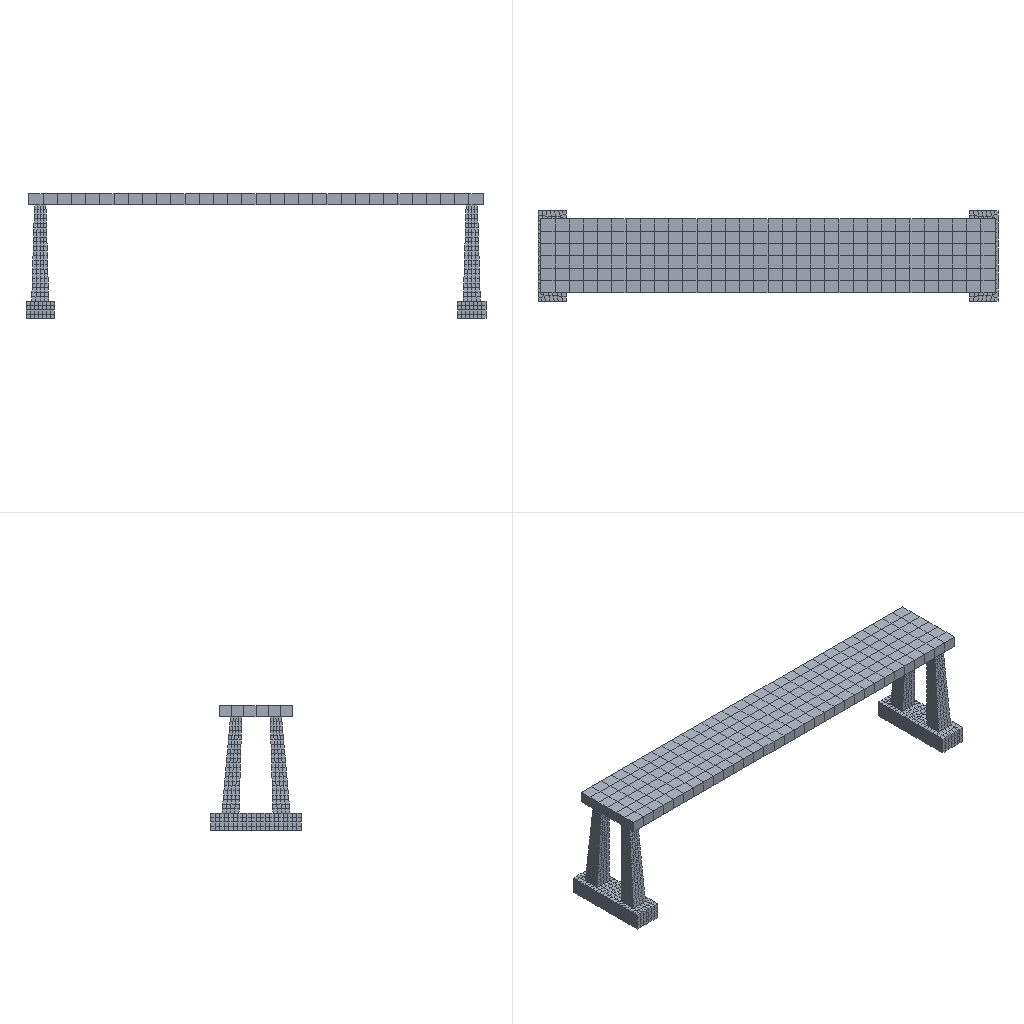Simulation study | ansys workbench
Set-up summary:
category,name,step,type,value,unit,region
solver,ansys_workbench
units,mm-N-s-tonne (MPa),,stated,"/units,MPA"
analysis,LS1,,static
load_step,LS1,LS1,static,nsubst=1; time=1
mesh,nodes,,,14374
mesh,elements,,,2852
element_type,SOLID186,,,2484
element_type,SURF154,,,192
element_type,TARGE170,,,88
element_type,CONTA174,,,88
material,steel,,E,210000,tonne s^-2 mm^-1
material,steel,,nu,0.3
material,steel,,density,7.85e-09,tonne mm^-3
load,Define Force Using Surface Effect Elements,LS1,surface-effect pres face 3,-0.09615,,SURF154 #8
bc,Fixed Supports,model,fixed,[dofs=ALL],,_FIXEDSU
contact,Contact Region,,bonded (always),element=CONTA174
contact,Contact Region 2,,bonded (always),element=CONTA174
named_set,_FIXEDSU,,node,821
Ansys APDL input file, long lists of numbers shortened:
/batch
/config,noeldb,1     ! force off writing results to database
*get,_wallstrt,active,,time,wall
! ANSYS input file written by Workbench version 2023 R1
! File used for geometry attach:
/title,wbnew--Static Structural (A5)
! ****** Begin Custom Load Command Snippet ******
/COM, ACT Extensions:
/COM,     LSDYNA, 2023.1
/COM,/COM,     ANSYSMotion, 2023.1
/COM,
! ****** End   Custom Load Command Snippet ******
*DIM,_wb_ProjectScratch_dir,string,248
_wb_ProjectScratch_dir(1) = ''
*DIM,_wb_SolverFiles_dir,string,248
_wb_SolverFiles_dir(1) = ''
*DIM,_wb_userfiles_dir,string,248
_wb_userfiles_dir(1) = ''
/com,--- Data in consistent NMM units. See Solving Units in the help system for more information.
/units,MPA
/nopr
/wb,file,start              !  signify a WB generated input file
/prep7
! Turn off shape checking because checks already performed inside WB mesher.
! See help system for more information.
SHPP,OFF,,NOWARN
/nolist
etcon,set             ! allow ANSYS to choose best KEYOP's for 180x elements, resets any applicable keyopt to MAPDL defaults
/com,*********** Nodes for the whole assembly ***********
nblock,3,,15811
(1i9,3e20.9e3)
        1     5.000000000E+02     1.450000000E+04     2.000000000E+04
! (14373 more lines like these left out)
-1
/wb,elem,start            !  set before creation of elements
/com,*********** Elements for Body 1 "longmendiao" ***********
et,1,186
keyo,1,2,1          ! set full integration on SOLID186
eblock,19,solid,,1148
(19i9)
        1        1        1        1        0        0        0        0       20        0      193     3225     3224     3193     3194     3322     3321     3290     3291
! (2295 more lines like these left out)
-1
/com,*********** Elements for Body 2 "longmendiao" ***********
et,2,186
keyo,2,2,1          ! set full integration on SOLID186
eblock,19,solid,,192
(19i9)
        2        2        2        2        0        0        0        0       20        0        1      393      459      461      395      394      460      462      396
! (383 more lines like these left out)
-1
/com,*********** Elements for Body 3 "longmendiao" ***********
et,3,186
keyo,3,2,1          ! set full integration on SOLID186
eblock,19,solid,,1144
(19i9)
        3        3        3        3        0        0        0        0       20        0     1341     9649     9648     9611     9610     9745     9744     9707     9706
! (2287 more lines like these left out)
-1
/wb,elem,end               !  done creating elements
/com,*********** Send User Defined Coordinate System(s) ***********
csys,0
toffst,273.15,  ! Temperature offset from absolute zero
/com,*********** Set Reference Temperature ***********
tref,22.
/wb,mat,start              !  starting to send materials
/com,*********** Send Materials ***********
MP,DENS,1,7.85e-09,	! tonne mm^-3
MP,EX,1,210000,	! tonne s^-2 mm^-1
MP,NUXY,1,0.3,
MP,DENS,2,7.85e-09,	! tonne mm^-3
MP,EX,2,210000,	! tonne s^-2 mm^-1
MP,NUXY,2,0.3,
MP,DENS,3,7.85e-09,	! tonne mm^-3
MP,EX,3,210000,	! tonne s^-2 mm^-1
MP,NUXY,3,0.3,
/wb,mat,end                !  done sending materials
!************************* Model Summary ********************
!longmendiao,	steel,	matid,	1
!longmendiao,	steel,	matid,	2
!longmendiao,	steel,	matid,	3
!************************* End Model Summary ********************
! get the diagonal of the bounding box. Needed later for other things
*get,_xmin,node,,mnloc,x
*get,_ymin,node,,mnloc,y
*get,_zmin,node,,mnloc,z
*get,_xmax,node,,mxloc,x
*get,_ymax,node,,mxloc,y
*get,_zmax,node,,mxloc,z
_ASMDIAG=(_xmax-_xmin)*(_xmax-_xmin)+(_ymax-_ymin)*(_ymax-_ymin)+(_zmax-_zmin)*(_zmax-_zmin)
_ASMDIAG=SQRT(_ASMDIAG)
/wb,contact,start          !  starting to send contact
/com,*********** Create Contact "Contact Region" ***********
/com,            Real Constant Set For Above Contact Is 5 & 4
*set,tid,5
*set,cid,4
r,tid
r,cid
et,tid,170
et,cid,174
eblock,10,,,32
(15i9)
     5195        5        5        5        0     2712     2691     2796     2817     6470     6675     3628     3674
! (31 more lines like these left out)
-1
eblock,10,,,32
(15i9)
     5227        4        4        4        0     2712     2691     2796     2817     6470     6675     3628     3674
! (31 more lines like these left out)
-1
eblock,10,,,12
(15i9)
     5259        4        5        4        0      459      393      395      461     1535     1442      616      604
! (11 more lines like these left out)
-1
eblock,10,,,12
(15i9)
     5271        5        4        5        0      459      393      395      461     1535     1442      616      604
! (11 more lines like these left out)
-1
keyo,cid,8,2               ! auto create asymmetric contact (from Program Controlled setting)
keyo,cid,10,0              ! adjust contact stiffness each NR iteration (from Program Controlled setting)
keyo,cid,12,5              ! bonded always
keyo,cid,18,1              ! small sliding turned on by application
keyo,cid,2,0               ! augmented Lagrange (from Program Controlled setting)
keyo,cid,4,0               ! on Gauss point (from Program Controlled setting)
keyo,cid,9,1               ! ignore initial gaps/penetration
keyo,cid,7,0               ! No Prediction
rmod,tid,3,10.      ! FKN
rmod,tid,5,0.       ! ICONT
rmod,tid,6,0.       ! PINB
rmod,tid,10,0.      ! CNOF
rmod,tid,12,0.      ! FKT
rmod,tid,36,33      ! WB DSID
rmod,cid,3,10.      ! FKN
rmod,cid,5,0.       ! ICONT
rmod,cid,6,0.       ! PINB
rmod,cid,10,0.      ! CNOF
rmod,cid,12,0.      ! FKT
rmod,cid,36,33      ! WB DSID
/com,*********** Create Contact "Contact Region 2" ***********
/com,            Real Constant Set For Above Contact Is 7 & 6
*set,tid,7
*set,cid,6
r,tid
r,cid
et,tid,170
et,cid,174
eblock,10,,,12
(15i9)
     5283        7        7        7        0      398      332      335      401     1445     1292     1448      574
! (11 more lines like these left out)
-1
eblock,10,,,12
(15i9)
     5295        6        6        6        0      398      332      335      401     1445     1292     1448      574
! (11 more lines like these left out)
-1
eblock,10,,,32
(15i9)
     5307        6        7        6        0     8614     8609     8610     8615    11650    11644     9774    10080
! (31 more lines like these left out)
-1
eblock,10,,,32
(15i9)
     5339        7        6        7        0     8614     8609     8610     8615    11650    11644     9774    10080
! (31 more lines like these left out)
-1
keyo,cid,8,2               ! auto create asymmetric contact (from Program Controlled setting)
keyo,cid,10,0              ! adjust contact stiffness each NR iteration (from Program Controlled setting)
keyo,cid,12,5              ! bonded always
keyo,cid,18,1              ! small sliding turned on by application
keyo,cid,2,0               ! augmented Lagrange (from Program Controlled setting)
keyo,cid,4,0               ! on Gauss point (from Program Controlled setting)
keyo,cid,9,1               ! ignore initial gaps/penetration
keyo,cid,7,0               ! No Prediction
rmod,tid,3,10.      ! FKN
rmod,tid,5,0.       ! ICONT
rmod,tid,6,0.       ! PINB
rmod,tid,10,0.      ! CNOF
rmod,tid,12,0.      ! FKT
rmod,tid,36,36      ! WB DSID
rmod,cid,3,10.      ! FKN
rmod,cid,5,0.       ! ICONT
rmod,cid,6,0.       ! PINB
rmod,cid,10,0.      ! CNOF
rmod,cid,12,0.      ! FKT
rmod,cid,36,36      ! WB DSID
nsel,all
esel,all
/wb,contact,end            !  done creating contacts
/golist
/wb,load,start             !  starting to send loads
/com,*********** Fixed Supports ***********
CMBLOCK,_FIXEDSU,NODE,      821
(8i10)
      1538      1539      1540      1541      1558      1559      1568      1569
! (102 more lines like these left out)
cmsel,s,_FIXEDSU
d,all,all
nsel,all
/com,*********** Define Force Using Surface Effect Elements ***********
local,12,0,0.,0.,0.,0.,0.,0.
csys,0
et,8,154
mat,8
eblock,10,,,192
(15i9)
     5371        8        8        8       12      396      394      460      462     1443     1537      571      610
! (191 more lines like these left out)
-1
esel,s,type,,8
keyop,8,2,1                ! Apply load in local coordinate system
keyop,8,7,1                ! Use original area so load is constant in large deformation
esel,all
/gst,on,on
fini
*get,_numnode,node,0,count
*get,_numelem,elem,0,count
*get, _MAXELEMNUM, elem, 0, NUM, MAX
*get, _MAXNODENUM, node, 0, NUM, MAX
*get, _MAXELEMTYPE, etyp, 0, NUM, MAX
*get, _MAXREALCONST, rcon, 0, NUM, MAX
/go
/wb,load,end               !  done creating loads
/com,--- Number of total nodes = %_numnode%
/com,--- Number of contact elements = 368
/com,--- Number of spring elements = 0
/com,--- Number of bearing elements = 0
/com,--- Number of solid elements = 2484
/com,--- Number of condensed parts = 0
/com,--- Number of total elements = %_numelem%
*get,_wallbsol,active,,time,wall
/com,****************************************************************************
/com,*************************    SOLUTION       ********************************
/com,****************************************************************************
/solu
antype,0                   ! static analysis
_thickRatio=  1     ! Ratio of thick parts in the model
eqsl,pcg,1e-8,,,,,,1
cntr,print,1               ! print out contact info and also make no initial contact an error
dmpoption,emat,no             ! Don't combine emat file for DANSYS
dmpoption,esav,no             ! Don't combine esav file for DANSYS
nldiag,cont,iter           ! print out contact info each equilibrium iteration
rescontrol,,none                 ! Do not keep any restart files
/com,****************************************************
/com,******************* SOLVE FOR LS 1 OF 1 ****************
esel,s,type,,8
nsle
sfe,all,1,pres,1,0.
sfe,all,2,pres,1,0.
sfe,all,3,pres,1,-9.61538461538533e-002
nsel,all
esel,all
/nopr
/gopr
nsub,1,1,1
time,1.
outres,erase
outres,all,none
outres,nsol,all,
outres,rsol,all
outres,eangl,all
outres,etmp,all
outres,veng,all
outres,strs,all,
outres,epel,all,
outres,eppl,all,
outres,cont,all,
! *********** WB SOLVE COMMAND ***********
! check interactive state
*get,ANSINTER_,active,,int
*if,ANSINTER_,ne,0,then
/eof
*endif
solve
/com *************** Write FE CONNECTORS *********
CEWRITE,file,ce,,INTE
/com,****************************************************
/com,*************** FINISHED SOLVE FOR LS 1 *************
*get,_wallasol,active,,time,wall
/nopr
*get,_numnode,node,0,count
*get,_numelem,elem,0,count
*get, _MAXELEMNUM, elem, 0, NUM, MAX
*get, _MAXNODENUM, node, 0, NUM, MAX,,,INTERNAL
*get, _MAXELEMTYPE, etyp, 0, NUM, MAX
*get, _MAXREALCONST, rcon, 0, NUM, MAX
*get,_NSOLTHREADS,active,0,ntfs
*get,_NSOLPROCESSES,active,0,npfs
/gopr
*get,_PCGITER,active,,solu,cgiter
/post1
xmlo,ENCODING,ISO-8859-1
xmlo,parm
/xml,parm,xml
fini
/gopr
*get,_walldone,active,,time,wall
_preptime=(_wallbsol-_wallstrt)*3600
_solvtime=(_wallasol-_wallbsol)*3600
_posttime=(_walldone-_wallasol)*3600
_totaltim=(_walldone-_wallstrt)*3600
*get,_dlbratio,active,0,solu,dlbr
*get,_combtime,active,0,solu,comb
*get,_ssmode,active,0,solu,ssmm
*get,_ndofs,active,0,solu,ndof
*get,_sol_end_time,active,0,set,time
*if,_sol_end_time,eq,1.,then
/fclean				!clean distributed files
*endif
/com,--- Total number of nodes = %_numnode%
/com,--- Total number of elements = %_numelem%
/com,--- Element load balance ratio = %_dlbratio%
/com,--- Time to combine distributed files = %_combtime%
/com,--- Sparse memory mode = %_ssmode%
/com,--- Number of DOF = %_ndofs%
/wb,file,end               ! done with WB generated input
Results summary:
result,analyses[0].index,,,1
result,analyses[0].system,,,SYS
result,analyses[0].deck,,,deck.dat
result,analyses[0].solve_status,,,completed
result,analyses[0].analysis_type,,,static
result,analyses[0].physics,,,mechanical
result,analyses[0].unit_system,,,"NMM: mm, ton, N, s, mV, mA, degC"
result,analyses[0].n_sets,,,1
result,analyses[0].load_steps[0].set,set=1,,1
result,analyses[0].load_steps[0].time_or_freq,set=1,,1
result,analyses[0].load_steps[0].max_displacement_magnitude,set=1,,105.404
result,analyses[0].load_steps[0].max_von_mises_nodal,set=1,,268.171
result,analyses[0].load_steps[0].reaction_force_sum_xyz[1],set=1,,0.1106
result,analyses[0].load_steps[0].reaction_force_sum_xyz[2],set=1,,-0.2626
result,analyses[0].load_steps[0].reaction_force_sum_xyz[3],set=1,,1e+08
result,geometry_export[0][0],,,.step
result,geometry_export[0][1],,,ok
result,geometry_export[0][2],,,3